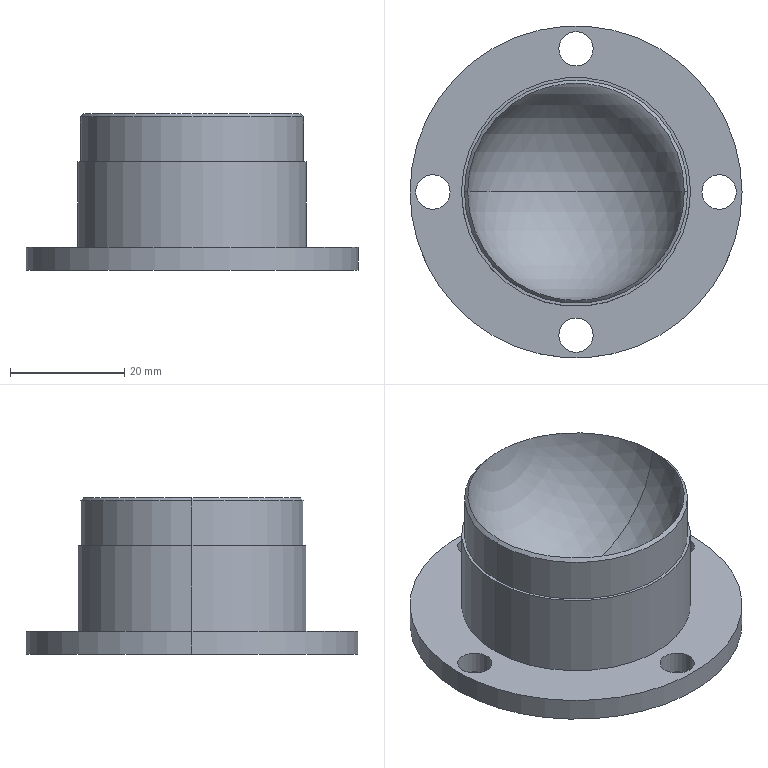Part | SolidWorks | features ICE 2, Extrusion 1, RevCut 1, StudWizard 1 | 1 solid | 21 faces | box 58 x 58 x 27.375 mm | volume 26425 mm3 | cylinder 14 | plane 3 | sphere 2 | cone 2 | commonest cylinder face diameters 6 x8 39 x2 40 x2 58 x2
STEP:
#1=CARTESIAN_POINT('',(-3.,25.,0.));
#2=VERTEX_POINT('',#1);
#3=CARTESIAN_POINT('',(3.,25.,0.));
#4=VERTEX_POINT('',#3);
#5=CARTESIAN_POINT('',(0.,25.,0.));
#6=DIRECTION('',(0.,0.,1.));
#7=DIRECTION('',(1.,0.,0.));
#8=AXIS2_PLACEMENT_3D('',#5,#6,#7);
#9=CIRCLE('',#8,3.);
#10=EDGE_CURVE('',#2,#4,#9,.T.);
#11=ORIENTED_EDGE('',*,*,#10,.F.);
#12=CARTESIAN_POINT('',(-3.,25.,4.));
#13=VERTEX_POINT('',#12);
#14=CARTESIAN_POINT('',(-3.,25.,-1.));
#15=DIRECTION('',(0.,0.,1.));
#16=VECTOR('',#15,1000.);
#17=LINE('',#14,#16);
#18=EDGE_CURVE('',#2,#13,#17,.T.);
#19=ORIENTED_EDGE('',*,*,#18,.T.);
#20=CARTESIAN_POINT('',(3.,25.,4.));
#21=VERTEX_POINT('',#20);
#22=CARTESIAN_POINT('',(0.,25.,4.));
#23=DIRECTION('',(0.,0.,1.));
#24=DIRECTION('',(1.,0.,0.));
#25=AXIS2_PLACEMENT_3D('',#22,#23,#24);
#26=CIRCLE('',#25,3.);
#27=EDGE_CURVE('',#13,#21,#26,.T.);
#28=ORIENTED_EDGE('',*,*,#27,.T.);
#29=CARTESIAN_POINT('',(3.,25.,-1.));
#30=DIRECTION('',(0.,0.,1.));
#31=VECTOR('',#30,1000.);
#32=LINE('',#29,#31);
#33=EDGE_CURVE('',#4,#21,#32,.T.);
#34=ORIENTED_EDGE('',*,*,#33,.F.);
#35=EDGE_LOOP('',(#11,#19,#28,#34));
#36=FACE_OUTER_BOUND('',#35,.T.);
#37=CARTESIAN_POINT('',(0.,25.,-1.));
#38=DIRECTION('',(0.,0.,1.));
#39=DIRECTION('',(1.,0.,0.));
#40=AXIS2_PLACEMENT_3D('',#37,#38,#39);
#41=CYLINDRICAL_SURFACE('',#40,3.);
#42=ADVANCED_FACE('',(#36),#41,.F.);
#43=CARTESIAN_POINT('',(22.,0.,0.));
#44=VERTEX_POINT('',#43);
#45=CARTESIAN_POINT('',(28.,0.,0.));
#46=VERTEX_POINT('',#45);
#47=CARTESIAN_POINT('',(25.,0.,0.));
#48=DIRECTION('',(0.,0.,1.));
#49=DIRECTION('',(1.,0.,0.));
#50=AXIS2_PLACEMENT_3D('',#47,#48,#49);
#51=CIRCLE('',#50,3.);
#52=EDGE_CURVE('',#44,#46,#51,.T.);
#53=ORIENTED_EDGE('',*,*,#52,.F.);
#54=CARTESIAN_POINT('',(22.,0.,4.));
#55=VERTEX_POINT('',#54);
#56=CARTESIAN_POINT('',(22.,0.,-1.));
#57=DIRECTION('',(0.,0.,1.));
#58=VECTOR('',#57,1000.);
#59=LINE('',#56,#58);
#60=EDGE_CURVE('',#44,#55,#59,.T.);
#61=ORIENTED_EDGE('',*,*,#60,.T.);
#62=CARTESIAN_POINT('',(28.,0.,4.));
#63=VERTEX_POINT('',#62);
#64=CARTESIAN_POINT('',(25.,0.,4.));
#65=DIRECTION('',(0.,0.,1.));
#66=DIRECTION('',(1.,0.,0.));
#67=AXIS2_PLACEMENT_3D('',#64,#65,#66);
#68=CIRCLE('',#67,3.);
#69=EDGE_CURVE('',#55,#63,#68,.T.);
#70=ORIENTED_EDGE('',*,*,#69,.T.);
#71=CARTESIAN_POINT('',(28.,0.,-1.));
#72=DIRECTION('',(0.,0.,1.));
#73=VECTOR('',#72,1000.);
#74=LINE('',#71,#73);
#75=EDGE_CURVE('',#46,#63,#74,.T.);
#76=ORIENTED_EDGE('',*,*,#75,.F.);
#77=EDGE_LOOP('',(#53,#61,#70,#76));
#78=FACE_OUTER_BOUND('',#77,.T.);
#79=CARTESIAN_POINT('',(25.,0.,-1.));
#80=DIRECTION('',(0.,0.,1.));
#81=DIRECTION('',(1.,0.,0.));
#82=AXIS2_PLACEMENT_3D('',#79,#80,#81);
#83=CYLINDRICAL_SURFACE('',#82,3.);
#84=ADVANCED_FACE('',(#78),#83,.F.);
#85=CARTESIAN_POINT('',(-3.,-25.,0.));
#86=VERTEX_POINT('',#85);
#87=CARTESIAN_POINT('',(3.,-25.,0.));
#88=VERTEX_POINT('',#87);
#89=CARTESIAN_POINT('',(0.,-25.,0.));
#90=DIRECTION('',(0.,0.,1.));
#91=DIRECTION('',(1.,0.,0.));
#92=AXIS2_PLACEMENT_3D('',#89,#90,#91);
#93=CIRCLE('',#92,3.);
#94=EDGE_CURVE('',#86,#88,#93,.T.);
#95=ORIENTED_EDGE('',*,*,#94,.F.);
#96=CARTESIAN_POINT('',(-3.,-25.,4.));
#97=VERTEX_POINT('',#96);
#98=CARTESIAN_POINT('',(-3.,-25.,-1.));
#99=DIRECTION('',(0.,0.,1.));
#100=VECTOR('',#99,1000.);
#101=LINE('',#98,#100);
#102=EDGE_CURVE('',#86,#97,#101,.T.);
#103=ORIENTED_EDGE('',*,*,#102,.T.);
#104=CARTESIAN_POINT('',(3.,-25.,4.));
#105=VERTEX_POINT('',#104);
#106=CARTESIAN_POINT('',(0.,-25.,4.));
#107=DIRECTION('',(0.,0.,1.));
#108=DIRECTION('',(1.,0.,0.));
#109=AXIS2_PLACEMENT_3D('',#106,#107,#108);
#110=CIRCLE('',#109,3.);
#111=EDGE_CURVE('',#97,#105,#110,.T.);
#112=ORIENTED_EDGE('',*,*,#111,.T.);
#113=CARTESIAN_POINT('',(3.,-25.,-1.));
#114=DIRECTION('',(0.,0.,1.));
#115=VECTOR('',#114,1000.);
#116=LINE('',#113,#115);
#117=EDGE_CURVE('',#88,#105,#116,.T.);
#118=ORIENTED_EDGE('',*,*,#117,.F.);
#119=EDGE_LOOP('',(#95,#103,#112,#118));
#120=FACE_OUTER_BOUND('',#119,.T.);
#121=CARTESIAN_POINT('',(0.,-25.,-1.));
#122=DIRECTION('',(0.,0.,1.));
#123=DIRECTION('',(1.,0.,0.));
#124=AXIS2_PLACEMENT_3D('',#121,#122,#123);
#125=CYLINDRICAL_SURFACE('',#124,3.);
#126=ADVANCED_FACE('',(#120),#125,.F.);
#127=CARTESIAN_POINT('',(-28.,0.,0.));
#128=VERTEX_POINT('',#127);
#129=CARTESIAN_POINT('',(-22.,0.,0.));
#130=VERTEX_POINT('',#129);
#131=CARTESIAN_POINT('',(-25.,0.,0.));
#132=DIRECTION('',(0.,0.,1.));
#133=DIRECTION('',(1.,0.,0.));
#134=AXIS2_PLACEMENT_3D('',#131,#132,#133);
#135=CIRCLE('',#134,3.);
#136=EDGE_CURVE('',#128,#130,#135,.T.);
#137=ORIENTED_EDGE('',*,*,#136,.F.);
#138=CARTESIAN_POINT('',(-28.,0.,4.));
#139=VERTEX_POINT('',#138);
#140=CARTESIAN_POINT('',(-28.,0.,-1.));
#141=DIRECTION('',(0.,0.,1.));
#142=VECTOR('',#141,1000.);
#143=LINE('',#140,#142);
#144=EDGE_CURVE('',#128,#139,#143,.T.);
#145=ORIENTED_EDGE('',*,*,#144,.T.);
#146=CARTESIAN_POINT('',(-22.,0.,4.));
#147=VERTEX_POINT('',#146);
#148=CARTESIAN_POINT('',(-25.,0.,4.));
#149=DIRECTION('',(0.,0.,1.));
#150=DIRECTION('',(1.,0.,0.));
#151=AXIS2_PLACEMENT_3D('',#148,#149,#150);
#152=CIRCLE('',#151,3.);
#153=EDGE_CURVE('',#139,#147,#152,.T.);
#154=ORIENTED_EDGE('',*,*,#153,.T.);
#155=CARTESIAN_POINT('',(-22.,0.,-1.));
#156=DIRECTION('',(0.,0.,1.));
#157=VECTOR('',#156,1000.);
#158=LINE('',#155,#157);
#159=EDGE_CURVE('',#130,#147,#158,.T.);
#160=ORIENTED_EDGE('',*,*,#159,.F.);
#161=EDGE_LOOP('',(#137,#145,#154,#160));
#162=FACE_OUTER_BOUND('',#161,.T.);
#163=CARTESIAN_POINT('',(-25.,0.,-1.));
#164=DIRECTION('',(0.,0.,1.));
#165=DIRECTION('',(1.,0.,0.));
#166=AXIS2_PLACEMENT_3D('',#163,#164,#165);
#167=CYLINDRICAL_SURFACE('',#166,3.);
#168=ADVANCED_FACE('',(#162),#167,.F.);
#169=CARTESIAN_POINT('',(18.93,0.,27.375));
#170=VERTEX_POINT('',#169);
#171=CARTESIAN_POINT('',(-18.93,0.,27.375));
#172=VERTEX_POINT('',#171);
#173=CARTESIAN_POINT('',(0.,0.,27.375));
#174=DIRECTION('',(0.,0.,-1.));
#175=DIRECTION('',(1.,0.,0.));
#176=AXIS2_PLACEMENT_3D('',#173,#174,#175);
#177=CIRCLE('',#176,18.93);
#178=EDGE_CURVE('',#170,#172,#177,.T.);
#179=ORIENTED_EDGE('',*,*,#178,.F.);
#180=CARTESIAN_POINT('',(0.,0.,29.));
#181=DIRECTION('',(0.,1.,0.));
#182=DIRECTION('',(0.,0.,1.));
#183=AXIS2_PLACEMENT_3D('',#180,#181,#182);
#184=CIRCLE('',#183,19.);
#185=EDGE_CURVE('',#170,#172,#184,.T.);
#186=ORIENTED_EDGE('',*,*,#185,.T.);
#187=EDGE_LOOP('',(#179,#186));
#188=FACE_OUTER_BOUND('',#187,.T.);
#189=CARTESIAN_POINT('',(0.,0.,29.));
#190=DIRECTION('',(0.,-1.,0.));
#191=DIRECTION('',(0.,0.,-1.));
#192=AXIS2_PLACEMENT_3D('',#189,#190,#191);
#193=SPHERICAL_SURFACE('',#192,19.);
#194=ADVANCED_FACE('',(#188),#193,.F.);
#195=CARTESIAN_POINT('',(0.,0.,27.375));
#196=DIRECTION('',(0.,0.,-1.));
#197=DIRECTION('',(1.,0.,0.));
#198=AXIS2_PLACEMENT_3D('',#195,#196,#197);
#199=CIRCLE('',#198,18.93);
#200=EDGE_CURVE('',#172,#170,#199,.T.);
#201=ORIENTED_EDGE('',*,*,#200,.T.);
#202=CARTESIAN_POINT('',(19.5,0.,26.805));
#203=VERTEX_POINT('',#202);
#204=CARTESIAN_POINT('',(17.305,0.,29.));
#205=DIRECTION('',(0.7071,0.,-0.7071));
#206=VECTOR('',#205,1000.);
#207=LINE('',#204,#206);
#208=EDGE_CURVE('',#170,#203,#207,.T.);
#209=ORIENTED_EDGE('',*,*,#208,.T.);
#210=CARTESIAN_POINT('',(-19.5,0.,26.805));
#211=VERTEX_POINT('',#210);
#212=CARTESIAN_POINT('',(0.,0.,26.805));
#213=DIRECTION('',(0.,0.,-1.));
#214=DIRECTION('',(-1.,0.,0.));
#215=AXIS2_PLACEMENT_3D('',#212,#213,#214);
#216=CIRCLE('',#215,19.5);
#217=EDGE_CURVE('',#211,#203,#216,.T.);
#218=ORIENTED_EDGE('',*,*,#217,.F.);
#219=CARTESIAN_POINT('',(-17.305,0.,29.));
#220=DIRECTION('',(-0.7071,0.,-0.7071));
#221=VECTOR('',#220,1000.);
#222=LINE('',#219,#221);
#223=EDGE_CURVE('',#172,#211,#222,.T.);
#224=ORIENTED_EDGE('',*,*,#223,.F.);
#225=EDGE_LOOP('',(#201,#209,#218,#224));
#226=FACE_OUTER_BOUND('',#225,.T.);
#227=CARTESIAN_POINT('',(0.,0.,29.));
#228=DIRECTION('',(0.,0.,-1.));
#229=DIRECTION('',(-1.,0.,0.));
#230=AXIS2_PLACEMENT_3D('',#227,#228,#229);
#231=CONICAL_SURFACE('',#230,17.305,0.7854);
#232=ADVANCED_FACE('',(#226),#231,.T.);
#233=ORIENTED_EDGE('',*,*,#217,.T.);
#234=CARTESIAN_POINT('',(19.5,0.,19.));
#235=VERTEX_POINT('',#234);
#236=CARTESIAN_POINT('',(19.5,0.,29.));
#237=DIRECTION('',(0.,0.,-1.));
#238=VECTOR('',#237,1000.);
#239=LINE('',#236,#238);
#240=EDGE_CURVE('',#203,#235,#239,.T.);
#241=ORIENTED_EDGE('',*,*,#240,.T.);
#242=CARTESIAN_POINT('',(-19.5,0.,19.));
#243=VERTEX_POINT('',#242);
#244=CARTESIAN_POINT('',(0.,0.,19.));
#245=DIRECTION('',(0.,0.,-1.));
#246=DIRECTION('',(-1.,0.,0.));
#247=AXIS2_PLACEMENT_3D('',#244,#245,#246);
#248=CIRCLE('',#247,19.5);
#249=EDGE_CURVE('',#243,#235,#248,.T.);
#250=ORIENTED_EDGE('',*,*,#249,.F.);
#251=CARTESIAN_POINT('',(-19.5,0.,29.));
#252=DIRECTION('',(0.,0.,-1.));
#253=VECTOR('',#252,1000.);
#254=LINE('',#251,#253);
#255=EDGE_CURVE('',#211,#243,#254,.T.);
#256=ORIENTED_EDGE('',*,*,#255,.F.);
#257=EDGE_LOOP('',(#233,#241,#250,#256));
#258=FACE_OUTER_BOUND('',#257,.T.);
#259=CARTESIAN_POINT('',(0.,0.,29.));
#260=DIRECTION('',(0.,0.,-1.));
#261=DIRECTION('',(-1.,0.,0.));
#262=AXIS2_PLACEMENT_3D('',#259,#260,#261);
#263=CYLINDRICAL_SURFACE('',#262,19.5);
#264=ADVANCED_FACE('',(#258),#263,.T.);
#265=CARTESIAN_POINT('',(-20.,0.,19.));
#266=VERTEX_POINT('',#265);
#267=CARTESIAN_POINT('',(20.,0.,19.));
#268=VERTEX_POINT('',#267);
#269=CARTESIAN_POINT('',(0.,0.,19.));
#270=DIRECTION('',(0.,0.,-1.));
#271=DIRECTION('',(-1.,0.,0.));
#272=AXIS2_PLACEMENT_3D('',#269,#270,#271);
#273=CIRCLE('',#272,20.);
#274=EDGE_CURVE('',#266,#268,#273,.T.);
#275=ORIENTED_EDGE('',*,*,#274,.T.);
#276=CARTESIAN_POINT('',(20.,0.,4.));
#277=VERTEX_POINT('',#276);
#278=CARTESIAN_POINT('',(20.,0.,29.));
#279=DIRECTION('',(0.,0.,-1.));
#280=VECTOR('',#279,1000.);
#281=LINE('',#278,#280);
#282=EDGE_CURVE('',#268,#277,#281,.T.);
#283=ORIENTED_EDGE('',*,*,#282,.T.);
#284=CARTESIAN_POINT('',(-20.,0.,4.));
#285=VERTEX_POINT('',#284);
#286=CARTESIAN_POINT('',(0.,0.,4.));
#287=DIRECTION('',(0.,0.,1.));
#288=DIRECTION('',(1.,0.,0.));
#289=AXIS2_PLACEMENT_3D('',#286,#287,#288);
#290=CIRCLE('',#289,20.);
#291=EDGE_CURVE('',#277,#285,#290,.T.);
#292=ORIENTED_EDGE('',*,*,#291,.T.);
#293=CARTESIAN_POINT('',(-20.,0.,29.));
#294=DIRECTION('',(0.,0.,-1.));
#295=VECTOR('',#294,1000.);
#296=LINE('',#293,#295);
#297=EDGE_CURVE('',#266,#285,#296,.T.);
#298=ORIENTED_EDGE('',*,*,#297,.F.);
#299=EDGE_LOOP('',(#275,#283,#292,#298));
#300=FACE_OUTER_BOUND('',#299,.T.);
#301=CARTESIAN_POINT('',(0.,0.,29.));
#302=DIRECTION('',(0.,0.,-1.));
#303=DIRECTION('',(-1.,0.,0.));
#304=AXIS2_PLACEMENT_3D('',#301,#302,#303);
#305=CYLINDRICAL_SURFACE('',#304,20.);
#306=ADVANCED_FACE('',(#300),#305,.T.);
#307=CARTESIAN_POINT('',(29.,0.,4.));
#308=VERTEX_POINT('',#307);
#309=CARTESIAN_POINT('',(-29.,0.,4.));
#310=VERTEX_POINT('',#309);
#311=CARTESIAN_POINT('',(0.,0.,4.));
#312=DIRECTION('',(0.,0.,1.));
#313=DIRECTION('',(1.,0.,0.));
#314=AXIS2_PLACEMENT_3D('',#311,#312,#313);
#315=CIRCLE('',#314,29.);
#316=EDGE_CURVE('',#308,#310,#315,.T.);
#317=ORIENTED_EDGE('',*,*,#316,.F.);
#318=CARTESIAN_POINT('',(29.,0.,0.));
#319=VERTEX_POINT('',#318);
#320=CARTESIAN_POINT('',(29.,0.,4.));
#321=DIRECTION('',(0.,0.,-1.));
#322=VECTOR('',#321,1000.);
#323=LINE('',#320,#322);
#324=EDGE_CURVE('',#308,#319,#323,.T.);
#325=ORIENTED_EDGE('',*,*,#324,.T.);
#326=CARTESIAN_POINT('',(-29.,0.,0.));
#327=VERTEX_POINT('',#326);
#328=CARTESIAN_POINT('',(0.,0.,0.));
#329=DIRECTION('',(0.,0.,1.));
#330=DIRECTION('',(1.,0.,0.));
#331=AXIS2_PLACEMENT_3D('',#328,#329,#330);
#332=CIRCLE('',#331,29.);
#333=EDGE_CURVE('',#319,#327,#332,.T.);
#334=ORIENTED_EDGE('',*,*,#333,.T.);
#335=CARTESIAN_POINT('',(-29.,0.,4.));
#336=DIRECTION('',(0.,0.,-1.));
#337=VECTOR('',#336,1000.);
#338=LINE('',#335,#337);
#339=EDGE_CURVE('',#310,#327,#338,.T.);
#340=ORIENTED_EDGE('',*,*,#339,.F.);
#341=EDGE_LOOP('',(#317,#325,#334,#340));
#342=FACE_OUTER_BOUND('',#341,.T.);
#343=CARTESIAN_POINT('',(0.,0.,4.));
#344=DIRECTION('',(0.,0.,-1.));
#345=DIRECTION('',(-1.,0.,0.));
#346=AXIS2_PLACEMENT_3D('',#343,#344,#345);
#347=CYLINDRICAL_SURFACE('',#346,29.);
#348=ADVANCED_FACE('',(#342),#347,.T.);
#349=ORIENTED_EDGE('',*,*,#324,.F.);
#350=CARTESIAN_POINT('',(0.,0.,4.));
#351=DIRECTION('',(0.,0.,1.));
#352=DIRECTION('',(1.,0.,0.));
#353=AXIS2_PLACEMENT_3D('',#350,#351,#352);
#354=CIRCLE('',#353,29.);
#355=EDGE_CURVE('',#310,#308,#354,.T.);
#356=ORIENTED_EDGE('',*,*,#355,.F.);
#357=ORIENTED_EDGE('',*,*,#339,.T.);
#358=CARTESIAN_POINT('',(0.,0.,0.));
#359=DIRECTION('',(0.,0.,1.));
#360=DIRECTION('',(1.,0.,0.));
#361=AXIS2_PLACEMENT_3D('',#358,#359,#360);
#362=CIRCLE('',#361,29.);
#363=EDGE_CURVE('',#327,#319,#362,.T.);
#364=ORIENTED_EDGE('',*,*,#363,.T.);
#365=EDGE_LOOP('',(#349,#356,#357,#364));
#366=FACE_OUTER_BOUND('',#365,.T.);
#367=CARTESIAN_POINT('',(0.,0.,4.));
#368=DIRECTION('',(0.,0.,-1.));
#369=DIRECTION('',(-1.,0.,0.));
#370=AXIS2_PLACEMENT_3D('',#367,#368,#369);
#371=CYLINDRICAL_SURFACE('',#370,29.);
#372=ADVANCED_FACE('',(#366),#371,.T.);
#373=CARTESIAN_POINT('',(0.,25.,4.));
#374=DIRECTION('',(0.,0.,1.));
#375=DIRECTION('',(1.,0.,0.));
#376=AXIS2_PLACEMENT_3D('',#373,#374,#375);
#377=CIRCLE('',#376,3.);
#378=EDGE_CURVE('',#21,#13,#377,.T.);
#379=ORIENTED_EDGE('',*,*,#378,.F.);
#380=ORIENTED_EDGE('',*,*,#27,.F.);
#381=EDGE_LOOP('',(#379,#380));
#382=FACE_BOUND('',#381,.T.);
#383=CARTESIAN_POINT('',(25.,0.,4.));
#384=DIRECTION('',(0.,0.,1.));
#385=DIRECTION('',(1.,0.,0.));
#386=AXIS2_PLACEMENT_3D('',#383,#384,#385);
#387=CIRCLE('',#386,3.);
#388=EDGE_CURVE('',#63,#55,#387,.T.);
#389=ORIENTED_EDGE('',*,*,#388,.F.);
#390=ORIENTED_EDGE('',*,*,#69,.F.);
#391=EDGE_LOOP('',(#389,#390));
#392=FACE_BOUND('',#391,.T.);
#393=CARTESIAN_POINT('',(0.,-25.,4.));
#394=DIRECTION('',(0.,0.,1.));
#395=DIRECTION('',(1.,0.,0.));
#396=AXIS2_PLACEMENT_3D('',#393,#394,#395);
#397=CIRCLE('',#396,3.);
#398=EDGE_CURVE('',#105,#97,#397,.T.);
#399=ORIENTED_EDGE('',*,*,#398,.F.);
#400=ORIENTED_EDGE('',*,*,#111,.F.);
#401=EDGE_LOOP('',(#399,#400));
#402=FACE_BOUND('',#401,.T.);
#403=CARTESIAN_POINT('',(-25.,0.,4.));
#404=DIRECTION('',(0.,0.,1.));
#405=DIRECTION('',(1.,0.,0.));
#406=AXIS2_PLACEMENT_3D('',#403,#404,#405);
#407=CIRCLE('',#406,3.);
#408=EDGE_CURVE('',#147,#139,#407,.T.);
#409=ORIENTED_EDGE('',*,*,#408,.F.);
#410=ORIENTED_EDGE('',*,*,#153,.F.);
#411=EDGE_LOOP('',(#409,#410));
#412=FACE_BOUND('',#411,.T.);
#413=CARTESIAN_POINT('',(0.,0.,4.));
#414=DIRECTION('',(0.,0.,1.));
#415=DIRECTION('',(1.,0.,0.));
#416=AXIS2_PLACEMENT_3D('',#413,#414,#415);
#417=CIRCLE('',#416,20.);
#418=EDGE_CURVE('',#285,#277,#417,.T.);
#419=ORIENTED_EDGE('',*,*,#418,.F.);
#420=ORIENTED_EDGE('',*,*,#291,.F.);
#421=EDGE_LOOP('',(#419,#420));
#422=FACE_BOUND('',#421,.T.);
#423=ORIENTED_EDGE('',*,*,#355,.T.);
#424=ORIENTED_EDGE('',*,*,#316,.T.);
#425=EDGE_LOOP('',(#423,#424));
#426=FACE_OUTER_BOUND('',#425,.T.);
#427=CARTESIAN_POINT('',(0.,0.,4.));
#428=DIRECTION('',(0.,0.,1.));
#429=DIRECTION('',(1.,0.,0.));
#430=AXIS2_PLACEMENT_3D('',#427,#428,#429);
#431=PLANE('',#430);
#432=ADVANCED_FACE('',(#382,#392,#402,#412,#422,#426),#431,.T.);
#433=CARTESIAN_POINT('',(0.,25.,0.));
#434=DIRECTION('',(0.,0.,1.));
#435=DIRECTION('',(1.,0.,0.));
#436=AXIS2_PLACEMENT_3D('',#433,#434,#435);
#437=CIRCLE('',#436,3.);
#438=EDGE_CURVE('',#4,#2,#437,.T.);
#439=ORIENTED_EDGE('',*,*,#438,.T.);
#440=ORIENTED_EDGE('',*,*,#10,.T.);
#441=EDGE_LOOP('',(#439,#440));
#442=FACE_BOUND('',#441,.T.);
#443=CARTESIAN_POINT('',(25.,0.,0.));
#444=DIRECTION('',(0.,0.,1.));
#445=DIRECTION('',(1.,0.,0.));
#446=AXIS2_PLACEMENT_3D('',#443,#444,#445);
#447=CIRCLE('',#446,3.);
#448=EDGE_CURVE('',#46,#44,#447,.T.);
#449=ORIENTED_EDGE('',*,*,#448,.T.);
#450=ORIENTED_EDGE('',*,*,#52,.T.);
#451=EDGE_LOOP('',(#449,#450));
#452=FACE_BOUND('',#451,.T.);
#453=CARTESIAN_POINT('',(0.,-25.,0.));
#454=DIRECTION('',(0.,0.,1.));
#455=DIRECTION('',(1.,0.,0.));
#456=AXIS2_PLACEMENT_3D('',#453,#454,#455);
#457=CIRCLE('',#456,3.);
#458=EDGE_CURVE('',#88,#86,#457,.T.);
#459=ORIENTED_EDGE('',*,*,#458,.T.);
#460=ORIENTED_EDGE('',*,*,#94,.T.);
#461=EDGE_LOOP('',(#459,#460));
#462=FACE_BOUND('',#461,.T.);
#463=CARTESIAN_POINT('',(-25.,0.,0.));
#464=DIRECTION('',(0.,0.,1.));
#465=DIRECTION('',(1.,0.,0.));
#466=AXIS2_PLACEMENT_3D('',#463,#464,#465);
#467=CIRCLE('',#466,3.);
#468=EDGE_CURVE('',#130,#128,#467,.T.);
#469=ORIENTED_EDGE('',*,*,#468,.T.);
#470=ORIENTED_EDGE('',*,*,#136,.T.);
#471=EDGE_LOOP('',(#469,#470));
#472=FACE_BOUND('',#471,.T.);
#473=ORIENTED_EDGE('',*,*,#363,.F.);
#474=ORIENTED_EDGE('',*,*,#333,.F.);
#475=EDGE_LOOP('',(#473,#474));
#476=FACE_OUTER_BOUND('',#475,.T.);
#477=CARTESIAN_POINT('',(0.,0.,0.));
#478=DIRECTION('',(0.,0.,1.));
#479=DIRECTION('',(1.,0.,0.));
#480=AXIS2_PLACEMENT_3D('',#477,#478,#479);
#481=PLANE('',#480);
#482=ADVANCED_FACE('',(#442,#452,#462,#472,#476),#481,.F.);
#483=ORIENTED_EDGE('',*,*,#282,.F.);
#484=CARTESIAN_POINT('',(0.,0.,19.));
#485=DIRECTION('',(0.,0.,-1.));
#486=DIRECTION('',(-1.,0.,0.));
#487=AXIS2_PLACEMENT_3D('',#484,#485,#486);
#488=CIRCLE('',#487,20.);
#489=EDGE_CURVE('',#268,#266,#488,.T.);
#490=ORIENTED_EDGE('',*,*,#489,.T.);
#491=ORIENTED_EDGE('',*,*,#297,.T.);
#492=ORIENTED_EDGE('',*,*,#418,.T.);
#493=EDGE_LOOP('',(#483,#490,#491,#492));
#494=FACE_OUTER_BOUND('',#493,.T.);
#495=CARTESIAN_POINT('',(0.,0.,29.));
#496=DIRECTION('',(0.,0.,-1.));
#497=DIRECTION('',(-1.,0.,0.));
#498=AXIS2_PLACEMENT_3D('',#495,#496,#497);
#499=CYLINDRICAL_SURFACE('',#498,20.);
#500=ADVANCED_FACE('',(#494),#499,.T.);
#501=ORIENTED_EDGE('',*,*,#240,.F.);
#502=CARTESIAN_POINT('',(0.,0.,26.805));
#503=DIRECTION('',(0.,0.,-1.));
#504=DIRECTION('',(-1.,0.,0.));
#505=AXIS2_PLACEMENT_3D('',#502,#503,#504);
#506=CIRCLE('',#505,19.5);
#507=EDGE_CURVE('',#203,#211,#506,.T.);
#508=ORIENTED_EDGE('',*,*,#507,.T.);
#509=ORIENTED_EDGE('',*,*,#255,.T.);
#510=CARTESIAN_POINT('',(0.,0.,19.));
#511=DIRECTION('',(0.,0.,-1.));
#512=DIRECTION('',(-1.,0.,0.));
#513=AXIS2_PLACEMENT_3D('',#510,#511,#512);
#514=CIRCLE('',#513,19.5);
#515=EDGE_CURVE('',#235,#243,#514,.T.);
#516=ORIENTED_EDGE('',*,*,#515,.F.);
#517=EDGE_LOOP('',(#501,#508,#509,#516));
#518=FACE_OUTER_BOUND('',#517,.T.);
#519=CARTESIAN_POINT('',(0.,0.,29.));
#520=DIRECTION('',(0.,0.,-1.));
#521=DIRECTION('',(-1.,0.,0.));
#522=AXIS2_PLACEMENT_3D('',#519,#520,#521);
#523=CYLINDRICAL_SURFACE('',#522,19.5);
#524=ADVANCED_FACE('',(#518),#523,.T.);
#525=ORIENTED_EDGE('',*,*,#274,.F.);
#526=ORIENTED_EDGE('',*,*,#489,.F.);
#527=EDGE_LOOP('',(#525,#526));
#528=FACE_OUTER_BOUND('',#527,.T.);
#529=ORIENTED_EDGE('',*,*,#249,.T.);
#530=ORIENTED_EDGE('',*,*,#515,.T.);
#531=EDGE_LOOP('',(#529,#530));
#532=FACE_BOUND('',#531,.T.);
#533=CARTESIAN_POINT('',(19.5,0.,19.));
#534=DIRECTION('',(0.,0.,-1.));
#535=DIRECTION('',(-1.,0.,0.));
#536=AXIS2_PLACEMENT_3D('',#533,#534,#535);
#537=PLANE('',#536);
#538=ADVANCED_FACE('',(#528,#532),#537,.F.);
#539=ORIENTED_EDGE('',*,*,#208,.F.);
#540=ORIENTED_EDGE('',*,*,#178,.T.);
#541=ORIENTED_EDGE('',*,*,#223,.T.);
#542=ORIENTED_EDGE('',*,*,#507,.F.);
#543=EDGE_LOOP('',(#539,#540,#541,#542));
#544=FACE_OUTER_BOUND('',#543,.T.);
#545=CARTESIAN_POINT('',(0.,0.,29.));
#546=DIRECTION('',(0.,0.,-1.));
#547=DIRECTION('',(-1.,0.,0.));
#548=AXIS2_PLACEMENT_3D('',#545,#546,#547);
#549=CONICAL_SURFACE('',#548,17.305,0.7854);
#550=ADVANCED_FACE('',(#544),#549,.T.);
#551=ORIENTED_EDGE('',*,*,#185,.F.);
#552=ORIENTED_EDGE('',*,*,#200,.F.);
#553=EDGE_LOOP('',(#551,#552));
#554=FACE_OUTER_BOUND('',#553,.T.);
#555=CARTESIAN_POINT('',(0.,0.,29.));
#556=DIRECTION('',(0.,-1.,0.));
#557=DIRECTION('',(0.,0.,-1.));
#558=AXIS2_PLACEMENT_3D('',#555,#556,#557);
#559=SPHERICAL_SURFACE('',#558,19.);
#560=ADVANCED_FACE('',(#554),#559,.F.);
#561=ORIENTED_EDGE('',*,*,#144,.F.);
#562=ORIENTED_EDGE('',*,*,#468,.F.);
#563=ORIENTED_EDGE('',*,*,#159,.T.);
#564=ORIENTED_EDGE('',*,*,#408,.T.);
#565=EDGE_LOOP('',(#561,#562,#563,#564));
#566=FACE_OUTER_BOUND('',#565,.T.);
#567=CARTESIAN_POINT('',(-25.,0.,-1.));
#568=DIRECTION('',(0.,0.,1.));
#569=DIRECTION('',(1.,0.,0.));
#570=AXIS2_PLACEMENT_3D('',#567,#568,#569);
#571=CYLINDRICAL_SURFACE('',#570,3.);
#572=ADVANCED_FACE('',(#566),#571,.F.);
#573=ORIENTED_EDGE('',*,*,#102,.F.);
#574=ORIENTED_EDGE('',*,*,#458,.F.);
#575=ORIENTED_EDGE('',*,*,#117,.T.);
#576=ORIENTED_EDGE('',*,*,#398,.T.);
#577=EDGE_LOOP('',(#573,#574,#575,#576));
#578=FACE_OUTER_BOUND('',#577,.T.);
#579=CARTESIAN_POINT('',(0.,-25.,-1.));
#580=DIRECTION('',(0.,0.,1.));
#581=DIRECTION('',(1.,0.,0.));
#582=AXIS2_PLACEMENT_3D('',#579,#580,#581);
#583=CYLINDRICAL_SURFACE('',#582,3.);
#584=ADVANCED_FACE('',(#578),#583,.F.);
#585=ORIENTED_EDGE('',*,*,#60,.F.);
#586=ORIENTED_EDGE('',*,*,#448,.F.);
#587=ORIENTED_EDGE('',*,*,#75,.T.);
#588=ORIENTED_EDGE('',*,*,#388,.T.);
#589=EDGE_LOOP('',(#585,#586,#587,#588));
#590=FACE_OUTER_BOUND('',#589,.T.);
#591=CARTESIAN_POINT('',(25.,0.,-1.));
#592=DIRECTION('',(0.,0.,1.));
#593=DIRECTION('',(1.,0.,0.));
#594=AXIS2_PLACEMENT_3D('',#591,#592,#593);
#595=CYLINDRICAL_SURFACE('',#594,3.);
#596=ADVANCED_FACE('',(#590),#595,.F.);
#597=ORIENTED_EDGE('',*,*,#18,.F.);
#598=ORIENTED_EDGE('',*,*,#438,.F.);
#599=ORIENTED_EDGE('',*,*,#33,.T.);
#600=ORIENTED_EDGE('',*,*,#378,.T.);
#601=EDGE_LOOP('',(#597,#598,#599,#600));
#602=FACE_OUTER_BOUND('',#601,.T.);
#603=CARTESIAN_POINT('',(0.,25.,-1.));
#604=DIRECTION('',(0.,0.,1.));
#605=DIRECTION('',(1.,0.,0.));
#606=AXIS2_PLACEMENT_3D('',#603,#604,#605);
#607=CYLINDRICAL_SURFACE('',#606,3.);
#608=ADVANCED_FACE('',(#602),#607,.F.);
#609=CLOSED_SHELL('',(#42,#84,#126,#168,#194,#232,#264,#306,#348,#372,#432,#482,#500,#524,#538,#550,#560,#572,#584,#596,#608));
#610=MANIFOLD_SOLID_BREP('',#609);
#611=CARTESIAN_POINT('',(0.,0.,0.));
#612=DIRECTION('',(0.,0.,1.));
#613=DIRECTION('',(1.,0.,0.));
#614=AXIS2_PLACEMENT_3D('',#611,#612,#613);
#615=(LENGTH_UNIT()NAMED_UNIT(*)SI_UNIT(.MILLI.,.METRE.));
#616=UNCERTAINTY_MEASURE_WITH_UNIT(LENGTH_MEASURE(0.00001),#615,'','');
#617=(NAMED_UNIT(*)PLANE_ANGLE_UNIT()SI_UNIT($,.RADIAN.));
#618=(NAMED_UNIT(*)SI_UNIT($,.STERADIAN.)SOLID_ANGLE_UNIT());
#619=(GEOMETRIC_REPRESENTATION_CONTEXT(3)GLOBAL_UNCERTAINTY_ASSIGNED_CONTEXT((#616))GLOBAL_UNIT_ASSIGNED_CONTEXT((#615,#617,#618))REPRESENTATION_CONTEXT('',''));
#620=ADVANCED_BREP_SHAPE_REPRESENTATION('',(#610,#614),#619);